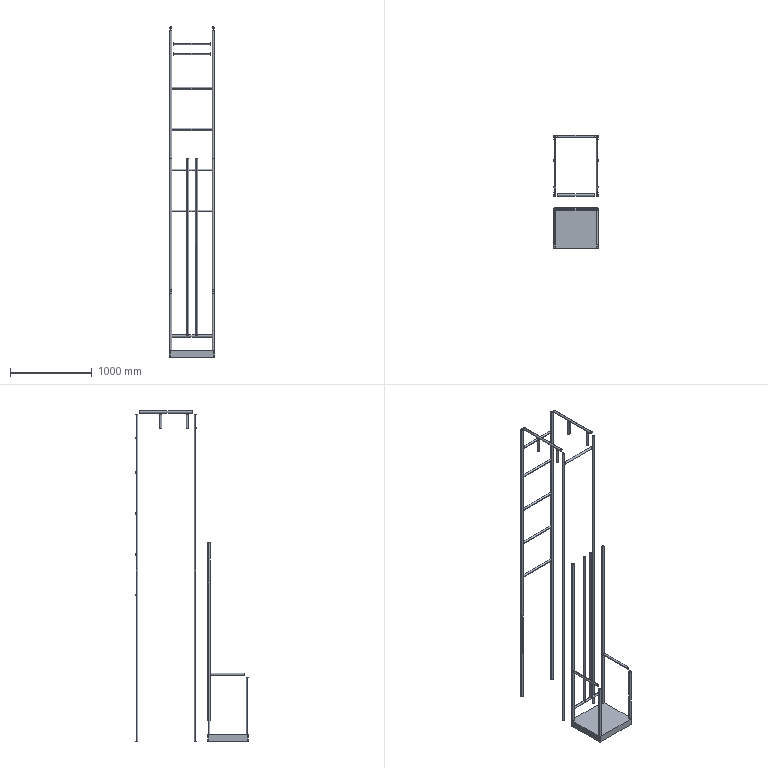Part | STEP file | FRAME ESTRUCTURA REV 3_Predeterminado<Como mecanizada> | 26 solids | 162 faces | box 552 x 1382 x 4049 mm | volume 25982334 mm3 | cylinder 104 | plane 58 | commonest cylinder face diameters 28.6 x54 26.2 x50